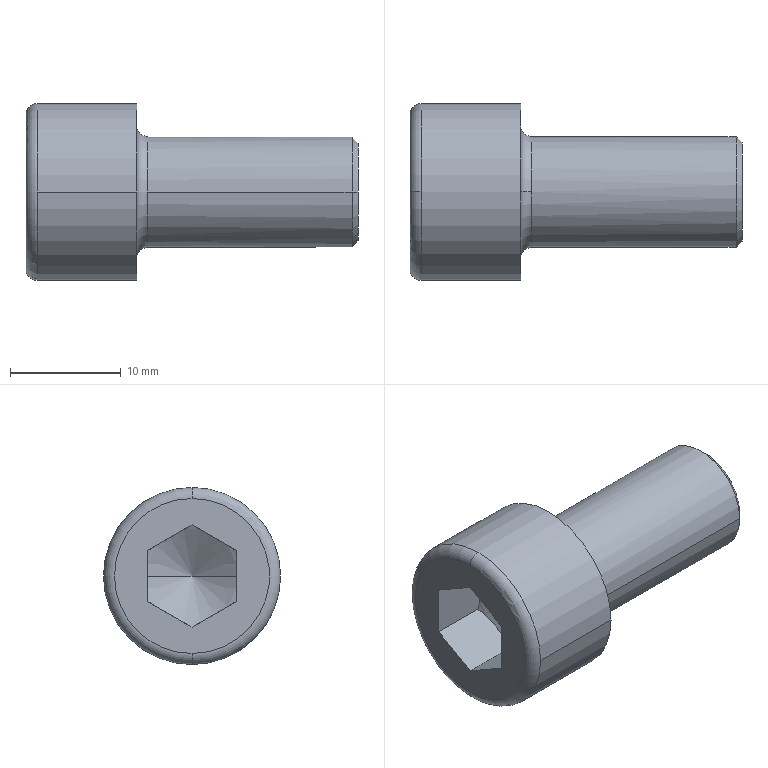Part | NX | features MOVE_FACE 6, BREP 1 | 1 solid | 21 faces | box 30 x 16 x 16 mm | volume 3238 mm3 | plane 9 | cylinder 4 | torus 4 | cone 4 | commonest cylinder face diameters 10 x2 16 x2
STEP:
#1=CARTESIAN_POINT('',(-9.,8.,0.));
#2=VERTEX_POINT('',#1);
#3=CARTESIAN_POINT('',(0.,8.,0.));
#4=VERTEX_POINT('',#3);
#5=CARTESIAN_POINT('',(-4.5,8.,0.));
#6=DIRECTION('',(1.,0.,0.));
#7=VECTOR('',#6,1000.);
#8=LINE('',#5,#7);
#9=EDGE_CURVE('',#2,#4,#8,.T.);
#10=ORIENTED_EDGE('',*,*,#9,.F.);
#11=CARTESIAN_POINT('',(-9.,0.,8.));
#12=VERTEX_POINT('',#11);
#13=CARTESIAN_POINT('',(-9.,0.,0.));
#14=DIRECTION('',(1.,0.,0.));
#15=DIRECTION('',(0.,1.,0.));
#16=AXIS2_PLACEMENT_3D('',#13,#14,#15);
#17=CIRCLE('',#16,8.);
#18=EDGE_CURVE('',#2,#12,#17,.T.);
#19=ORIENTED_EDGE('',*,*,#18,.T.);
#20=CARTESIAN_POINT('',(-9.,-8.,0.));
#21=VERTEX_POINT('',#20);
#22=CARTESIAN_POINT('',(-9.,0.,0.));
#23=DIRECTION('',(1.,0.,0.));
#24=DIRECTION('',(0.,1.,0.));
#25=AXIS2_PLACEMENT_3D('',#22,#23,#24);
#26=CIRCLE('',#25,8.);
#27=EDGE_CURVE('',#12,#21,#26,.T.);
#28=ORIENTED_EDGE('',*,*,#27,.T.);
#29=CARTESIAN_POINT('',(0.,-8.,0.));
#30=VERTEX_POINT('',#29);
#31=CARTESIAN_POINT('',(-4.5,-8.,0.));
#32=DIRECTION('',(-1.,0.,0.));
#33=VECTOR('',#32,1000.);
#34=LINE('',#31,#33);
#35=EDGE_CURVE('',#30,#21,#34,.T.);
#36=ORIENTED_EDGE('',*,*,#35,.F.);
#37=CARTESIAN_POINT('',(0.,0.,0.));
#38=DIRECTION('',(1.,0.,0.));
#39=DIRECTION('',(0.,1.,0.));
#40=AXIS2_PLACEMENT_3D('',#37,#38,#39);
#41=CIRCLE('',#40,8.);
#42=EDGE_CURVE('',#4,#30,#41,.T.);
#43=ORIENTED_EDGE('',*,*,#42,.F.);
#44=EDGE_LOOP('',(#10,#19,#28,#36,#43));
#45=FACE_BOUND('',#44,.T.);
#46=CARTESIAN_POINT('',(-4.5,0.,0.));
#47=DIRECTION('',(1.,0.,0.));
#48=DIRECTION('',(0.,-1.,0.));
#49=AXIS2_PLACEMENT_3D('',#46,#47,#48);
#50=CYLINDRICAL_SURFACE('',#49,8.);
#51=ADVANCED_FACE('',(#45),#50,.T.);
#52=CARTESIAN_POINT('',(-10.,0.,-7.));
#53=VERTEX_POINT('',#52);
#54=CARTESIAN_POINT('',(-9.,0.,-8.));
#55=VERTEX_POINT('',#54);
#56=CARTESIAN_POINT('',(-9.,0.,-7.));
#57=DIRECTION('',(0.,-1.,0.));
#58=DIRECTION('',(0.,0.,-1.));
#59=AXIS2_PLACEMENT_3D('',#56,#57,#58);
#60=CIRCLE('',#59,1.);
#61=EDGE_CURVE('',#53,#55,#60,.T.);
#62=ORIENTED_EDGE('',*,*,#61,.F.);
#63=CARTESIAN_POINT('',(-10.,7.,0.));
#64=VERTEX_POINT('',#63);
#65=CARTESIAN_POINT('',(-10.,0.,0.));
#66=DIRECTION('',(1.,0.,0.));
#67=DIRECTION('',(0.,1.,0.));
#68=AXIS2_PLACEMENT_3D('',#65,#66,#67);
#69=CIRCLE('',#68,7.);
#70=EDGE_CURVE('',#53,#64,#69,.T.);
#71=ORIENTED_EDGE('',*,*,#70,.T.);
#72=CARTESIAN_POINT('',(-10.,0.,7.));
#73=VERTEX_POINT('',#72);
#74=CARTESIAN_POINT('',(-10.,0.,0.));
#75=DIRECTION('',(1.,0.,0.));
#76=DIRECTION('',(0.,1.,0.));
#77=AXIS2_PLACEMENT_3D('',#74,#75,#76);
#78=CIRCLE('',#77,7.);
#79=EDGE_CURVE('',#64,#73,#78,.T.);
#80=ORIENTED_EDGE('',*,*,#79,.T.);
#81=CARTESIAN_POINT('',(-9.,0.,7.));
#82=DIRECTION('',(0.,-1.,0.));
#83=DIRECTION('',(0.,0.,1.));
#84=AXIS2_PLACEMENT_3D('',#81,#82,#83);
#85=CIRCLE('',#84,1.);
#86=EDGE_CURVE('',#12,#73,#85,.T.);
#87=ORIENTED_EDGE('',*,*,#86,.F.);
#88=ORIENTED_EDGE('',*,*,#18,.F.);
#89=CARTESIAN_POINT('',(-9.,0.,0.));
#90=DIRECTION('',(1.,0.,0.));
#91=DIRECTION('',(0.,1.,0.));
#92=AXIS2_PLACEMENT_3D('',#89,#90,#91);
#93=CIRCLE('',#92,8.);
#94=EDGE_CURVE('',#55,#2,#93,.T.);
#95=ORIENTED_EDGE('',*,*,#94,.F.);
#96=EDGE_LOOP('',(#62,#71,#80,#87,#88,#95));
#97=FACE_BOUND('',#96,.T.);
#98=CARTESIAN_POINT('',(-9.,0.,0.));
#99=DIRECTION('',(1.,0.,0.));
#100=DIRECTION('',(0.,0.,1.));
#101=AXIS2_PLACEMENT_3D('',#98,#99,#100);
#102=TOROIDAL_SURFACE('',#101,7.,1.);
#103=ADVANCED_FACE('',(#97),#102,.T.);
#104=CARTESIAN_POINT('',(19.459,5.,0.));
#105=VERTEX_POINT('',#104);
#106=CARTESIAN_POINT('',(20.,4.459,0.));
#107=VERTEX_POINT('',#106);
#108=CARTESIAN_POINT('',(19.729,4.729,0.));
#109=DIRECTION('',(0.7071,-0.7071,0.));
#110=VECTOR('',#109,1000.);
#111=LINE('',#108,#110);
#112=EDGE_CURVE('',#105,#107,#111,.T.);
#113=ORIENTED_EDGE('',*,*,#112,.F.);
#114=CARTESIAN_POINT('',(19.459,-5.,0.));
#115=VERTEX_POINT('',#114);
#116=CARTESIAN_POINT('',(19.459,0.,0.));
#117=DIRECTION('',(1.,0.,0.));
#118=DIRECTION('',(0.,1.,0.));
#119=AXIS2_PLACEMENT_3D('',#116,#117,#118);
#120=CIRCLE('',#119,5.);
#121=EDGE_CURVE('',#105,#115,#120,.T.);
#122=ORIENTED_EDGE('',*,*,#121,.T.);
#123=CARTESIAN_POINT('',(20.,-4.459,0.));
#124=VERTEX_POINT('',#123);
#125=CARTESIAN_POINT('',(19.729,-4.729,0.));
#126=DIRECTION('',(-0.7071,-0.7071,0.));
#127=VECTOR('',#126,1000.);
#128=LINE('',#125,#127);
#129=EDGE_CURVE('',#124,#115,#128,.T.);
#130=ORIENTED_EDGE('',*,*,#129,.F.);
#131=CARTESIAN_POINT('',(20.,0.,0.));
#132=DIRECTION('',(1.,0.,0.));
#133=DIRECTION('',(0.,1.,0.));
#134=AXIS2_PLACEMENT_3D('',#131,#132,#133);
#135=CIRCLE('',#134,4.459);
#136=EDGE_CURVE('',#107,#124,#135,.T.);
#137=ORIENTED_EDGE('',*,*,#136,.F.);
#138=EDGE_LOOP('',(#113,#122,#130,#137));
#139=FACE_BOUND('',#138,.T.);
#140=CARTESIAN_POINT('',(19.729,0.,0.));
#141=DIRECTION('',(-1.,0.,0.));
#142=DIRECTION('',(0.,-1.,0.));
#143=AXIS2_PLACEMENT_3D('',#140,#141,#142);
#144=CONICAL_SURFACE('',#143,4.729,0.7854);
#145=ADVANCED_FACE('',(#139),#144,.T.);
#146=CARTESIAN_POINT('',(1.,5.,0.));
#147=VERTEX_POINT('',#146);
#148=CARTESIAN_POINT('',(8.229,5.,0.));
#149=DIRECTION('',(1.,0.,0.));
#150=VECTOR('',#149,1000.);
#151=LINE('',#148,#150);
#152=EDGE_CURVE('',#147,#105,#151,.T.);
#153=ORIENTED_EDGE('',*,*,#152,.F.);
#154=CARTESIAN_POINT('',(1.,0.,5.));
#155=VERTEX_POINT('',#154);
#156=CARTESIAN_POINT('',(1.,0.,0.));
#157=DIRECTION('',(1.,0.,0.));
#158=DIRECTION('',(0.,1.,0.));
#159=AXIS2_PLACEMENT_3D('',#156,#157,#158);
#160=CIRCLE('',#159,5.);
#161=EDGE_CURVE('',#147,#155,#160,.T.);
#162=ORIENTED_EDGE('',*,*,#161,.T.);
#163=CARTESIAN_POINT('',(1.,-5.,0.));
#164=VERTEX_POINT('',#163);
#165=CARTESIAN_POINT('',(1.,0.,0.));
#166=DIRECTION('',(1.,0.,0.));
#167=DIRECTION('',(0.,1.,0.));
#168=AXIS2_PLACEMENT_3D('',#165,#166,#167);
#169=CIRCLE('',#168,5.);
#170=EDGE_CURVE('',#155,#164,#169,.T.);
#171=ORIENTED_EDGE('',*,*,#170,.T.);
#172=CARTESIAN_POINT('',(8.229,-5.,0.));
#173=DIRECTION('',(-1.,0.,0.));
#174=VECTOR('',#173,1000.);
#175=LINE('',#172,#174);
#176=EDGE_CURVE('',#115,#164,#175,.T.);
#177=ORIENTED_EDGE('',*,*,#176,.F.);
#178=ORIENTED_EDGE('',*,*,#121,.F.);
#179=EDGE_LOOP('',(#153,#162,#171,#177,#178));
#180=FACE_BOUND('',#179,.T.);
#181=CARTESIAN_POINT('',(8.229,0.,0.));
#182=DIRECTION('',(1.,0.,0.));
#183=DIRECTION('',(0.,-1.,0.));
#184=AXIS2_PLACEMENT_3D('',#181,#182,#183);
#185=CYLINDRICAL_SURFACE('',#184,5.);
#186=ADVANCED_FACE('',(#180),#185,.T.);
#187=CARTESIAN_POINT('',(0.,0.,6.));
#188=VERTEX_POINT('',#187);
#189=CARTESIAN_POINT('',(1.,0.,6.));
#190=DIRECTION('',(0.,-1.,0.));
#191=DIRECTION('',(0.,0.,1.));
#192=AXIS2_PLACEMENT_3D('',#189,#190,#191);
#193=CIRCLE('',#192,1.);
#194=EDGE_CURVE('',#188,#155,#193,.T.);
#195=ORIENTED_EDGE('',*,*,#194,.F.);
#196=CARTESIAN_POINT('',(0.,0.,-6.));
#197=VERTEX_POINT('',#196);
#198=CARTESIAN_POINT('',(0.,0.,0.));
#199=DIRECTION('',(1.,0.,0.));
#200=DIRECTION('',(0.,1.,0.));
#201=AXIS2_PLACEMENT_3D('',#198,#199,#200);
#202=CIRCLE('',#201,6.);
#203=EDGE_CURVE('',#188,#197,#202,.T.);
#204=ORIENTED_EDGE('',*,*,#203,.T.);
#205=CARTESIAN_POINT('',(1.,0.,-5.));
#206=VERTEX_POINT('',#205);
#207=CARTESIAN_POINT('',(1.,0.,-6.));
#208=DIRECTION('',(0.,-1.,0.));
#209=DIRECTION('',(0.,0.,-1.));
#210=AXIS2_PLACEMENT_3D('',#207,#208,#209);
#211=CIRCLE('',#210,1.);
#212=EDGE_CURVE('',#206,#197,#211,.T.);
#213=ORIENTED_EDGE('',*,*,#212,.F.);
#214=CARTESIAN_POINT('',(1.,0.,0.));
#215=DIRECTION('',(1.,0.,0.));
#216=DIRECTION('',(0.,1.,0.));
#217=AXIS2_PLACEMENT_3D('',#214,#215,#216);
#218=CIRCLE('',#217,5.);
#219=EDGE_CURVE('',#164,#206,#218,.T.);
#220=ORIENTED_EDGE('',*,*,#219,.F.);
#221=ORIENTED_EDGE('',*,*,#170,.F.);
#222=EDGE_LOOP('',(#195,#204,#213,#220,#221));
#223=FACE_BOUND('',#222,.T.);
#224=CARTESIAN_POINT('',(1.,0.,0.));
#225=DIRECTION('',(1.,0.,0.));
#226=DIRECTION('',(0.,0.,1.));
#227=AXIS2_PLACEMENT_3D('',#224,#225,#226);
#228=TOROIDAL_SURFACE('',#227,6.,1.);
#229=ADVANCED_FACE('',(#223),#228,.F.);
#230=CARTESIAN_POINT('',(-4.644,-4.001,0.));
#231=VERTEX_POINT('',#230);
#232=CARTESIAN_POINT('',(-2.334,0.,0.));
#233=VERTEX_POINT('',#232);
#234=CARTESIAN_POINT('',(-3.667,-2.31,0.));
#235=DIRECTION('',(0.5,0.866,0.));
#236=VECTOR('',#235,1000.);
#237=LINE('',#234,#236);
#238=EDGE_CURVE('',#231,#233,#237,.T.);
#239=ORIENTED_EDGE('',*,*,#238,.T.);
#240=CARTESIAN_POINT('',(-4.644,4.001,0.));
#241=VERTEX_POINT('',#240);
#242=CARTESIAN_POINT('',(-3.667,2.31,0.));
#243=DIRECTION('',(-0.5,0.866,0.));
#244=VECTOR('',#243,1000.);
#245=LINE('',#242,#244);
#246=EDGE_CURVE('',#233,#241,#245,.T.);
#247=ORIENTED_EDGE('',*,*,#246,.T.);
#248=CARTESIAN_POINT('',(-5.001,4.001,-2.31));
#249=VERTEX_POINT('',#248);
#250=CARTESIAN_POINT('',(-5.001,4.001,2.31));
#251=CARTESIAN_POINT('',(-4.334,4.001,0.));
#252=CARTESIAN_POINT('',(-5.001,4.001,-2.31));
#253=(BOUNDED_CURVE()B_SPLINE_CURVE(2,(#250,#251,#252),.UNSPECIFIED.,.F.,.F.)B_SPLINE_CURVE_WITH_KNOTS((3,3),(0.,1.),.PIECEWISE_BEZIER_KNOTS.)CURVE()GEOMETRIC_REPRESENTATION_ITEM()RATIONAL_B_SPLINE_CURVE((1.,1.155,1.))REPRESENTATION_ITEM(''));
#254=EDGE_CURVE('',#241,#249,#253,.T.);
#255=ORIENTED_EDGE('',*,*,#254,.T.);
#256=CARTESIAN_POINT('',(-5.001,0.,-4.62));
#257=VERTEX_POINT('',#256);
#258=CARTESIAN_POINT('',(-5.001,4.001,-2.31));
#259=CARTESIAN_POINT('',(-4.334,2.001,-3.465));
#260=CARTESIAN_POINT('',(-5.001,0.,-4.62));
#261=(BOUNDED_CURVE()B_SPLINE_CURVE(2,(#258,#259,#260),.UNSPECIFIED.,.F.,.F.)B_SPLINE_CURVE_WITH_KNOTS((3,3),(0.,1.),.PIECEWISE_BEZIER_KNOTS.)CURVE()GEOMETRIC_REPRESENTATION_ITEM()RATIONAL_B_SPLINE_CURVE((1.,1.155,1.))REPRESENTATION_ITEM(''));
#262=EDGE_CURVE('',#249,#257,#261,.T.);
#263=ORIENTED_EDGE('',*,*,#262,.T.);
#264=CARTESIAN_POINT('',(-5.001,-4.001,-2.31));
#265=VERTEX_POINT('',#264);
#266=CARTESIAN_POINT('',(-5.001,0.,-4.62));
#267=CARTESIAN_POINT('',(-4.334,-2.001,-3.465));
#268=CARTESIAN_POINT('',(-5.001,-4.001,-2.31));
#269=(BOUNDED_CURVE()B_SPLINE_CURVE(2,(#266,#267,#268),.UNSPECIFIED.,.F.,.F.)B_SPLINE_CURVE_WITH_KNOTS((3,3),(0.,1.),.PIECEWISE_BEZIER_KNOTS.)CURVE()GEOMETRIC_REPRESENTATION_ITEM()RATIONAL_B_SPLINE_CURVE((1.,1.155,1.))REPRESENTATION_ITEM(''));
#270=EDGE_CURVE('',#257,#265,#269,.T.);
#271=ORIENTED_EDGE('',*,*,#270,.T.);
#272=CARTESIAN_POINT('',(-5.001,-4.001,-2.31));
#273=CARTESIAN_POINT('',(-4.334,-4.001,0.));
#274=CARTESIAN_POINT('',(-5.001,-4.001,2.31));
#275=(BOUNDED_CURVE()B_SPLINE_CURVE(2,(#272,#273,#274),.UNSPECIFIED.,.F.,.F.)B_SPLINE_CURVE_WITH_KNOTS((3,3),(0.,1.),.PIECEWISE_BEZIER_KNOTS.)CURVE()GEOMETRIC_REPRESENTATION_ITEM()RATIONAL_B_SPLINE_CURVE((1.,1.155,1.))REPRESENTATION_ITEM(''));
#276=EDGE_CURVE('',#265,#231,#275,.T.);
#277=ORIENTED_EDGE('',*,*,#276,.T.);
#278=EDGE_LOOP('',(#239,#247,#255,#263,#271,#277));
#279=FACE_BOUND('',#278,.T.);
#280=CARTESIAN_POINT('',(-3.667,0.,0.));
#281=DIRECTION('',(-1.,0.,0.));
#282=DIRECTION('',(0.,-1.,0.));
#283=AXIS2_PLACEMENT_3D('',#280,#281,#282);
#284=CONICAL_SURFACE('',#283,2.31,1.047);
#285=ADVANCED_FACE('',(#279),#284,.F.);
#286=CARTESIAN_POINT('',(-10.,-4.001,-2.31));
#287=VERTEX_POINT('',#286);
#288=CARTESIAN_POINT('',(-10.,0.,-4.62));
#289=VERTEX_POINT('',#288);
#290=CARTESIAN_POINT('',(-10.,-0.688,-4.223));
#291=DIRECTION('',(0.,0.866,-0.5));
#292=VECTOR('',#291,1000.);
#293=LINE('',#290,#292);
#294=EDGE_CURVE('',#287,#289,#293,.T.);
#295=ORIENTED_EDGE('',*,*,#294,.F.);
#296=CARTESIAN_POINT('',(-7.501,-4.001,-2.31));
#297=DIRECTION('',(-1.,0.,0.));
#298=VECTOR('',#297,1000.);
#299=LINE('',#296,#298);
#300=EDGE_CURVE('',#265,#287,#299,.T.);
#301=ORIENTED_EDGE('',*,*,#300,.F.);
#302=ORIENTED_EDGE('',*,*,#270,.F.);
#303=CARTESIAN_POINT('',(-7.501,0.,-4.62));
#304=DIRECTION('',(-1.,0.,0.));
#305=VECTOR('',#304,1000.);
#306=LINE('',#303,#305);
#307=EDGE_CURVE('',#257,#289,#306,.T.);
#308=ORIENTED_EDGE('',*,*,#307,.T.);
#309=EDGE_LOOP('',(#295,#301,#302,#308));
#310=FACE_BOUND('',#309,.T.);
#311=CARTESIAN_POINT('',(-10.001,-2.001,-3.465));
#312=DIRECTION('',(0.,-0.5,-0.866));
#313=DIRECTION('',(0.,-0.866,0.5));
#314=AXIS2_PLACEMENT_3D('',#311,#312,#313);
#315=PLANE('',#314);
#316=ADVANCED_FACE('',(#310),#315,.F.);
#317=CARTESIAN_POINT('',(-10.,4.001,-2.31));
#318=VERTEX_POINT('',#317);
#319=CARTESIAN_POINT('',(-10.,3.313,-2.707));
#320=DIRECTION('',(0.,0.866,0.5));
#321=VECTOR('',#320,1000.);
#322=LINE('',#319,#321);
#323=EDGE_CURVE('',#289,#318,#322,.T.);
#324=ORIENTED_EDGE('',*,*,#323,.F.);
#325=ORIENTED_EDGE('',*,*,#307,.F.);
#326=ORIENTED_EDGE('',*,*,#262,.F.);
#327=CARTESIAN_POINT('',(-7.501,4.001,-2.31));
#328=DIRECTION('',(-1.,0.,0.));
#329=VECTOR('',#328,1000.);
#330=LINE('',#327,#329);
#331=EDGE_CURVE('',#249,#318,#330,.T.);
#332=ORIENTED_EDGE('',*,*,#331,.T.);
#333=EDGE_LOOP('',(#324,#325,#326,#332));
#334=FACE_BOUND('',#333,.T.);
#335=CARTESIAN_POINT('',(-10.001,2.001,-3.465));
#336=DIRECTION('',(0.,0.5,-0.866));
#337=DIRECTION('',(0.,-0.866,-0.5));
#338=AXIS2_PLACEMENT_3D('',#335,#336,#337);
#339=PLANE('',#338);
#340=ADVANCED_FACE('',(#334),#339,.F.);
#341=CARTESIAN_POINT('',(-10.,4.001,2.31));
#342=VERTEX_POINT('',#341);
#343=CARTESIAN_POINT('',(-10.,4.001,0.));
#344=DIRECTION('',(0.,0.,1.));
#345=VECTOR('',#344,1000.);
#346=LINE('',#343,#345);
#347=EDGE_CURVE('',#318,#342,#346,.T.);
#348=ORIENTED_EDGE('',*,*,#347,.F.);
#349=ORIENTED_EDGE('',*,*,#331,.F.);
#350=ORIENTED_EDGE('',*,*,#254,.F.);
#351=CARTESIAN_POINT('',(-5.001,4.001,2.31));
#352=VERTEX_POINT('',#351);
#353=CARTESIAN_POINT('',(-5.001,4.001,2.31));
#354=CARTESIAN_POINT('',(-4.334,4.001,0.));
#355=CARTESIAN_POINT('',(-5.001,4.001,-2.31));
#356=(BOUNDED_CURVE()B_SPLINE_CURVE(2,(#353,#354,#355),.UNSPECIFIED.,.F.,.F.)B_SPLINE_CURVE_WITH_KNOTS((3,3),(0.,1.),.PIECEWISE_BEZIER_KNOTS.)CURVE()GEOMETRIC_REPRESENTATION_ITEM()RATIONAL_B_SPLINE_CURVE((1.,1.155,1.))REPRESENTATION_ITEM(''));
#357=EDGE_CURVE('',#352,#241,#356,.T.);
#358=ORIENTED_EDGE('',*,*,#357,.F.);
#359=CARTESIAN_POINT('',(-7.501,4.001,2.31));
#360=DIRECTION('',(-1.,0.,0.));
#361=VECTOR('',#360,1000.);
#362=LINE('',#359,#361);
#363=EDGE_CURVE('',#352,#342,#362,.T.);
#364=ORIENTED_EDGE('',*,*,#363,.T.);
#365=EDGE_LOOP('',(#348,#349,#350,#358,#364));
#366=FACE_BOUND('',#365,.T.);
#367=CARTESIAN_POINT('',(-10.001,4.001,0.));
#368=DIRECTION('',(0.,1.,0.));
#369=DIRECTION('',(0.,0.,-1.));
#370=AXIS2_PLACEMENT_3D('',#367,#368,#369);
#371=PLANE('',#370);
#372=ADVANCED_FACE('',(#366),#371,.F.);
#373=CARTESIAN_POINT('',(-10.,-4.001,2.31));
#374=VERTEX_POINT('',#373);
#375=CARTESIAN_POINT('',(-10.,-4.001,0.));
#376=DIRECTION('',(0.,0.,-1.));
#377=VECTOR('',#376,1000.);
#378=LINE('',#375,#377);
#379=EDGE_CURVE('',#374,#287,#378,.T.);
#380=ORIENTED_EDGE('',*,*,#379,.F.);
#381=CARTESIAN_POINT('',(-5.001,-4.001,2.31));
#382=VERTEX_POINT('',#381);
#383=CARTESIAN_POINT('',(-7.501,-4.001,2.31));
#384=DIRECTION('',(-1.,0.,0.));
#385=VECTOR('',#384,1000.);
#386=LINE('',#383,#385);
#387=EDGE_CURVE('',#382,#374,#386,.T.);
#388=ORIENTED_EDGE('',*,*,#387,.F.);
#389=CARTESIAN_POINT('',(-5.001,-4.001,-2.31));
#390=CARTESIAN_POINT('',(-4.334,-4.001,0.));
#391=CARTESIAN_POINT('',(-5.001,-4.001,2.31));
#392=(BOUNDED_CURVE()B_SPLINE_CURVE(2,(#389,#390,#391),.UNSPECIFIED.,.F.,.F.)B_SPLINE_CURVE_WITH_KNOTS((3,3),(0.,1.),.PIECEWISE_BEZIER_KNOTS.)CURVE()GEOMETRIC_REPRESENTATION_ITEM()RATIONAL_B_SPLINE_CURVE((1.,1.155,1.))REPRESENTATION_ITEM(''));
#393=EDGE_CURVE('',#231,#382,#392,.T.);
#394=ORIENTED_EDGE('',*,*,#393,.F.);
#395=ORIENTED_EDGE('',*,*,#276,.F.);
#396=ORIENTED_EDGE('',*,*,#300,.T.);
#397=EDGE_LOOP('',(#380,#388,#394,#395,#396));
#398=FACE_BOUND('',#397,.T.);
#399=CARTESIAN_POINT('',(-10.001,-4.001,0.));
#400=DIRECTION('',(0.,-1.,0.));
#401=DIRECTION('',(0.,0.,1.));
#402=AXIS2_PLACEMENT_3D('',#399,#400,#401);
#403=PLANE('',#402);
#404=ADVANCED_FACE('',(#398),#403,.F.);
#405=CARTESIAN_POINT('',(-10.,0.,4.62));
#406=VERTEX_POINT('',#405);
#407=CARTESIAN_POINT('',(-10.,3.313,2.707));
#408=DIRECTION('',(0.,-0.866,0.5));
#409=VECTOR('',#408,1000.);
#410=LINE('',#407,#409);
#411=EDGE_CURVE('',#342,#406,#410,.T.);
#412=ORIENTED_EDGE('',*,*,#411,.F.);
#413=ORIENTED_EDGE('',*,*,#363,.F.);
#414=CARTESIAN_POINT('',(-5.001,0.,4.62));
#415=VERTEX_POINT('',#414);
#416=CARTESIAN_POINT('',(-5.001,0.,4.62));
#417=CARTESIAN_POINT('',(-4.334,2.001,3.465));
#418=CARTESIAN_POINT('',(-5.001,4.001,2.31));
#419=(BOUNDED_CURVE()B_SPLINE_CURVE(2,(#416,#417,#418),.UNSPECIFIED.,.F.,.F.)B_SPLINE_CURVE_WITH_KNOTS((3,3),(0.,1.),.PIECEWISE_BEZIER_KNOTS.)CURVE()GEOMETRIC_REPRESENTATION_ITEM()RATIONAL_B_SPLINE_CURVE((1.,1.155,1.))REPRESENTATION_ITEM(''));
#420=EDGE_CURVE('',#415,#352,#419,.T.);
#421=ORIENTED_EDGE('',*,*,#420,.F.);
#422=CARTESIAN_POINT('',(-7.501,0.,4.62));
#423=DIRECTION('',(1.,0.,0.));
#424=VECTOR('',#423,1000.);
#425=LINE('',#422,#424);
#426=EDGE_CURVE('',#406,#415,#425,.T.);
#427=ORIENTED_EDGE('',*,*,#426,.F.);
#428=EDGE_LOOP('',(#412,#413,#421,#427));
#429=FACE_BOUND('',#428,.T.);
#430=CARTESIAN_POINT('',(-10.001,2.001,3.465));
#431=DIRECTION('',(0.,0.5,0.866));
#432=DIRECTION('',(0.,0.866,-0.5));
#433=AXIS2_PLACEMENT_3D('',#430,#431,#432);
#434=PLANE('',#433);
#435=ADVANCED_FACE('',(#429),#434,.F.);
#436=CARTESIAN_POINT('',(-10.,-0.688,4.223));
#437=DIRECTION('',(0.,-0.866,-0.5));
#438=VECTOR('',#437,1000.);
#439=LINE('',#436,#438);
#440=EDGE_CURVE('',#406,#374,#439,.T.);
#441=ORIENTED_EDGE('',*,*,#440,.F.);
#442=ORIENTED_EDGE('',*,*,#426,.T.);
#443=CARTESIAN_POINT('',(-5.001,-4.001,2.31));
#444=CARTESIAN_POINT('',(-4.334,-2.001,3.465));
#445=CARTESIAN_POINT('',(-5.001,0.,4.62));
#446=(BOUNDED_CURVE()B_SPLINE_CURVE(2,(#443,#444,#445),.UNSPECIFIED.,.F.,.F.)B_SPLINE_CURVE_WITH_KNOTS((3,3),(0.,1.),.PIECEWISE_BEZIER_KNOTS.)CURVE()GEOMETRIC_REPRESENTATION_ITEM()RATIONAL_B_SPLINE_CURVE((1.,1.155,1.))REPRESENTATION_ITEM(''));
#447=EDGE_CURVE('',#382,#415,#446,.T.);
#448=ORIENTED_EDGE('',*,*,#447,.F.);
#449=ORIENTED_EDGE('',*,*,#387,.T.);
#450=EDGE_LOOP('',(#441,#442,#448,#449));
#451=FACE_BOUND('',#450,.T.);
#452=CARTESIAN_POINT('',(-10.001,-2.001,3.465));
#453=DIRECTION('',(0.,-0.5,0.866));
#454=DIRECTION('',(0.,0.866,0.5));
#455=AXIS2_PLACEMENT_3D('',#452,#453,#454);
#456=PLANE('',#455);
#457=ADVANCED_FACE('',(#451),#456,.F.);
#458=ORIENTED_EDGE('',*,*,#238,.F.);
#459=ORIENTED_EDGE('',*,*,#393,.T.);
#460=ORIENTED_EDGE('',*,*,#447,.T.);
#461=ORIENTED_EDGE('',*,*,#420,.T.);
#462=ORIENTED_EDGE('',*,*,#357,.T.);
#463=ORIENTED_EDGE('',*,*,#246,.F.);
#464=EDGE_LOOP('',(#458,#459,#460,#461,#462,#463));
#465=FACE_BOUND('',#464,.T.);
#466=CARTESIAN_POINT('',(-3.667,0.,0.));
#467=DIRECTION('',(-1.,0.,0.));
#468=DIRECTION('',(0.,-1.,0.));
#469=AXIS2_PLACEMENT_3D('',#466,#467,#468);
#470=CONICAL_SURFACE('',#469,2.31,1.047);
#471=ADVANCED_FACE('',(#465),#470,.F.);
#472=ORIENTED_EDGE('',*,*,#194,.T.);
#473=ORIENTED_EDGE('',*,*,#161,.F.);
#474=CARTESIAN_POINT('',(1.,0.,0.));
#475=DIRECTION('',(1.,0.,0.));
#476=DIRECTION('',(0.,1.,0.));
#477=AXIS2_PLACEMENT_3D('',#474,#475,#476);
#478=CIRCLE('',#477,5.);
#479=EDGE_CURVE('',#206,#147,#478,.T.);
#480=ORIENTED_EDGE('',*,*,#479,.F.);
#481=ORIENTED_EDGE('',*,*,#212,.T.);
#482=CARTESIAN_POINT('',(0.,6.,0.));
#483=VERTEX_POINT('',#482);
#484=CARTESIAN_POINT('',(0.,0.,0.));
#485=DIRECTION('',(1.,0.,0.));
#486=DIRECTION('',(0.,1.,0.));
#487=AXIS2_PLACEMENT_3D('',#484,#485,#486);
#488=CIRCLE('',#487,6.);
#489=EDGE_CURVE('',#197,#483,#488,.T.);
#490=ORIENTED_EDGE('',*,*,#489,.T.);
#491=CARTESIAN_POINT('',(0.,0.,0.));
#492=DIRECTION('',(1.,0.,0.));
#493=DIRECTION('',(0.,1.,0.));
#494=AXIS2_PLACEMENT_3D('',#491,#492,#493);
#495=CIRCLE('',#494,6.);
#496=EDGE_CURVE('',#483,#188,#495,.T.);
#497=ORIENTED_EDGE('',*,*,#496,.T.);
#498=EDGE_LOOP('',(#472,#473,#480,#481,#490,#497));
#499=FACE_BOUND('',#498,.T.);
#500=CARTESIAN_POINT('',(1.,0.,0.));
#501=DIRECTION('',(1.,0.,0.));
#502=DIRECTION('',(0.,0.,1.));
#503=AXIS2_PLACEMENT_3D('',#500,#501,#502);
#504=TOROIDAL_SURFACE('',#503,6.,1.);
#505=ADVANCED_FACE('',(#499),#504,.F.);
#506=ORIENTED_EDGE('',*,*,#152,.T.);
#507=CARTESIAN_POINT('',(19.459,0.,0.));
#508=DIRECTION('',(1.,0.,0.));
#509=DIRECTION('',(0.,1.,0.));
#510=AXIS2_PLACEMENT_3D('',#507,#508,#509);
#511=CIRCLE('',#510,5.);
#512=EDGE_CURVE('',#115,#105,#511,.T.);
#513=ORIENTED_EDGE('',*,*,#512,.F.);
#514=ORIENTED_EDGE('',*,*,#176,.T.);
#515=ORIENTED_EDGE('',*,*,#219,.T.);
#516=ORIENTED_EDGE('',*,*,#479,.T.);
#517=EDGE_LOOP('',(#506,#513,#514,#515,#516));
#518=FACE_BOUND('',#517,.T.);
#519=CARTESIAN_POINT('',(8.229,0.,0.));
#520=DIRECTION('',(1.,0.,0.));
#521=DIRECTION('',(0.,-1.,0.));
#522=AXIS2_PLACEMENT_3D('',#519,#520,#521);
#523=CYLINDRICAL_SURFACE('',#522,5.);
#524=ADVANCED_FACE('',(#518),#523,.T.);
#525=ORIENTED_EDGE('',*,*,#112,.T.);
#526=CARTESIAN_POINT('',(20.,0.,0.));
#527=DIRECTION('',(1.,0.,0.));
#528=DIRECTION('',(0.,1.,0.));
#529=AXIS2_PLACEMENT_3D('',#526,#527,#528);
#530=CIRCLE('',#529,4.459);
#531=EDGE_CURVE('',#124,#107,#530,.T.);
#532=ORIENTED_EDGE('',*,*,#531,.F.);
#533=ORIENTED_EDGE('',*,*,#129,.T.);
#534=ORIENTED_EDGE('',*,*,#512,.T.);
#535=EDGE_LOOP('',(#525,#532,#533,#534));
#536=FACE_BOUND('',#535,.T.);
#537=CARTESIAN_POINT('',(19.729,0.,0.));
#538=DIRECTION('',(-1.,0.,0.));
#539=DIRECTION('',(0.,-1.,0.));
#540=AXIS2_PLACEMENT_3D('',#537,#538,#539);
#541=CONICAL_SURFACE('',#540,4.729,0.7854);
#542=ADVANCED_FACE('',(#536),#541,.T.);
#543=ORIENTED_EDGE('',*,*,#136,.T.);
#544=ORIENTED_EDGE('',*,*,#531,.T.);
#545=EDGE_LOOP('',(#543,#544));
#546=FACE_BOUND('',#545,.T.);
#547=CARTESIAN_POINT('',(20.,2.229,0.));
#548=DIRECTION('',(1.,0.,0.));
#549=DIRECTION('',(0.,-1.,0.));
#550=AXIS2_PLACEMENT_3D('',#547,#548,#549);
#551=PLANE('',#550);
#552=ADVANCED_FACE('',(#546),#551,.T.);
#553=ORIENTED_EDGE('',*,*,#411,.T.);
#554=ORIENTED_EDGE('',*,*,#440,.T.);
#555=ORIENTED_EDGE('',*,*,#379,.T.);
#556=ORIENTED_EDGE('',*,*,#294,.T.);
#557=ORIENTED_EDGE('',*,*,#323,.T.);
#558=ORIENTED_EDGE('',*,*,#347,.T.);
#559=EDGE_LOOP('',(#553,#554,#555,#556,#557,#558));
#560=FACE_BOUND('',#559,.T.);
#561=ORIENTED_EDGE('',*,*,#79,.F.);
#562=ORIENTED_EDGE('',*,*,#70,.F.);
#563=CARTESIAN_POINT('',(-10.,0.,0.));
#564=DIRECTION('',(1.,0.,0.));
#565=DIRECTION('',(0.,1.,0.));
#566=AXIS2_PLACEMENT_3D('',#563,#564,#565);
#567=CIRCLE('',#566,7.);
#568=EDGE_CURVE('',#73,#53,#567,.T.);
#569=ORIENTED_EDGE('',*,*,#568,.F.);
#570=EDGE_LOOP('',(#561,#562,#569));
#571=FACE_BOUND('',#570,.T.);
#572=CARTESIAN_POINT('',(-10.,3.5,0.));
#573=DIRECTION('',(-1.,0.,0.));
#574=DIRECTION('',(0.,1.,0.));
#575=AXIS2_PLACEMENT_3D('',#572,#573,#574);
#576=PLANE('',#575);
#577=ADVANCED_FACE('',(#560,#571),#576,.T.);
#578=ORIENTED_EDGE('',*,*,#61,.T.);
#579=CARTESIAN_POINT('',(-9.,0.,0.));
#580=DIRECTION('',(1.,0.,0.));
#581=DIRECTION('',(0.,1.,0.));
#582=AXIS2_PLACEMENT_3D('',#579,#580,#581);
#583=CIRCLE('',#582,8.);
#584=EDGE_CURVE('',#21,#55,#583,.T.);
#585=ORIENTED_EDGE('',*,*,#584,.F.);
#586=ORIENTED_EDGE('',*,*,#27,.F.);
#587=ORIENTED_EDGE('',*,*,#86,.T.);
#588=ORIENTED_EDGE('',*,*,#568,.T.);
#589=EDGE_LOOP('',(#578,#585,#586,#587,#588));
#590=FACE_BOUND('',#589,.T.);
#591=CARTESIAN_POINT('',(-9.,0.,0.));
#592=DIRECTION('',(1.,0.,0.));
#593=DIRECTION('',(0.,0.,1.));
#594=AXIS2_PLACEMENT_3D('',#591,#592,#593);
#595=TOROIDAL_SURFACE('',#594,7.,1.);
#596=ADVANCED_FACE('',(#590),#595,.T.);
#597=ORIENTED_EDGE('',*,*,#9,.T.);
#598=CARTESIAN_POINT('',(0.,0.,0.));
#599=DIRECTION('',(1.,0.,0.));
#600=DIRECTION('',(0.,1.,0.));
#601=AXIS2_PLACEMENT_3D('',#598,#599,#600);
#602=CIRCLE('',#601,8.);
#603=EDGE_CURVE('',#30,#4,#602,.T.);
#604=ORIENTED_EDGE('',*,*,#603,.F.);
#605=ORIENTED_EDGE('',*,*,#35,.T.);
#606=ORIENTED_EDGE('',*,*,#584,.T.);
#607=ORIENTED_EDGE('',*,*,#94,.T.);
#608=EDGE_LOOP('',(#597,#604,#605,#606,#607));
#609=FACE_BOUND('',#608,.T.);
#610=CARTESIAN_POINT('',(-4.5,0.,0.));
#611=DIRECTION('',(1.,0.,0.));
#612=DIRECTION('',(0.,-1.,0.));
#613=AXIS2_PLACEMENT_3D('',#610,#611,#612);
#614=CYLINDRICAL_SURFACE('',#613,8.);
#615=ADVANCED_FACE('',(#609),#614,.T.);
#616=ORIENTED_EDGE('',*,*,#496,.F.);
#617=ORIENTED_EDGE('',*,*,#489,.F.);
#618=ORIENTED_EDGE('',*,*,#203,.F.);
#619=EDGE_LOOP('',(#616,#617,#618));
#620=FACE_BOUND('',#619,.T.);
#621=ORIENTED_EDGE('',*,*,#42,.T.);
#622=ORIENTED_EDGE('',*,*,#603,.T.);
#623=EDGE_LOOP('',(#621,#622));
#624=FACE_BOUND('',#623,.T.);
#625=CARTESIAN_POINT('',(0.,7.,0.));
#626=DIRECTION('',(1.,0.,0.));
#627=DIRECTION('',(0.,-1.,0.));
#628=AXIS2_PLACEMENT_3D('',#625,#626,#627);
#629=PLANE('',#628);
#630=ADVANCED_FACE('',(#620,#624),#629,.T.);
#631=CLOSED_SHELL('',(#51,#103,#145,#186,#229,#285,#316,#340,#372,#404,#435,#457,#471,#505,#524,#542,#552,#577,#596,#615,#630));
#632=MANIFOLD_SOLID_BREP('',#631);
#633=(LENGTH_UNIT()NAMED_UNIT(*)SI_UNIT(.MILLI.,.METRE.));
#634=UNCERTAINTY_MEASURE_WITH_UNIT(LENGTH_MEASURE(0.00001),#633,'','');
#635=(NAMED_UNIT(*)PLANE_ANGLE_UNIT()SI_UNIT($,.RADIAN.));
#636=(NAMED_UNIT(*)SI_UNIT($,.STERADIAN.)SOLID_ANGLE_UNIT());
#637=(GEOMETRIC_REPRESENTATION_CONTEXT(3)GLOBAL_UNCERTAINTY_ASSIGNED_CONTEXT((#634))GLOBAL_UNIT_ASSIGNED_CONTEXT((#633,#635,#636))REPRESENTATION_CONTEXT('',''));
#638=ADVANCED_BREP_SHAPE_REPRESENTATION('',(#632),#637);